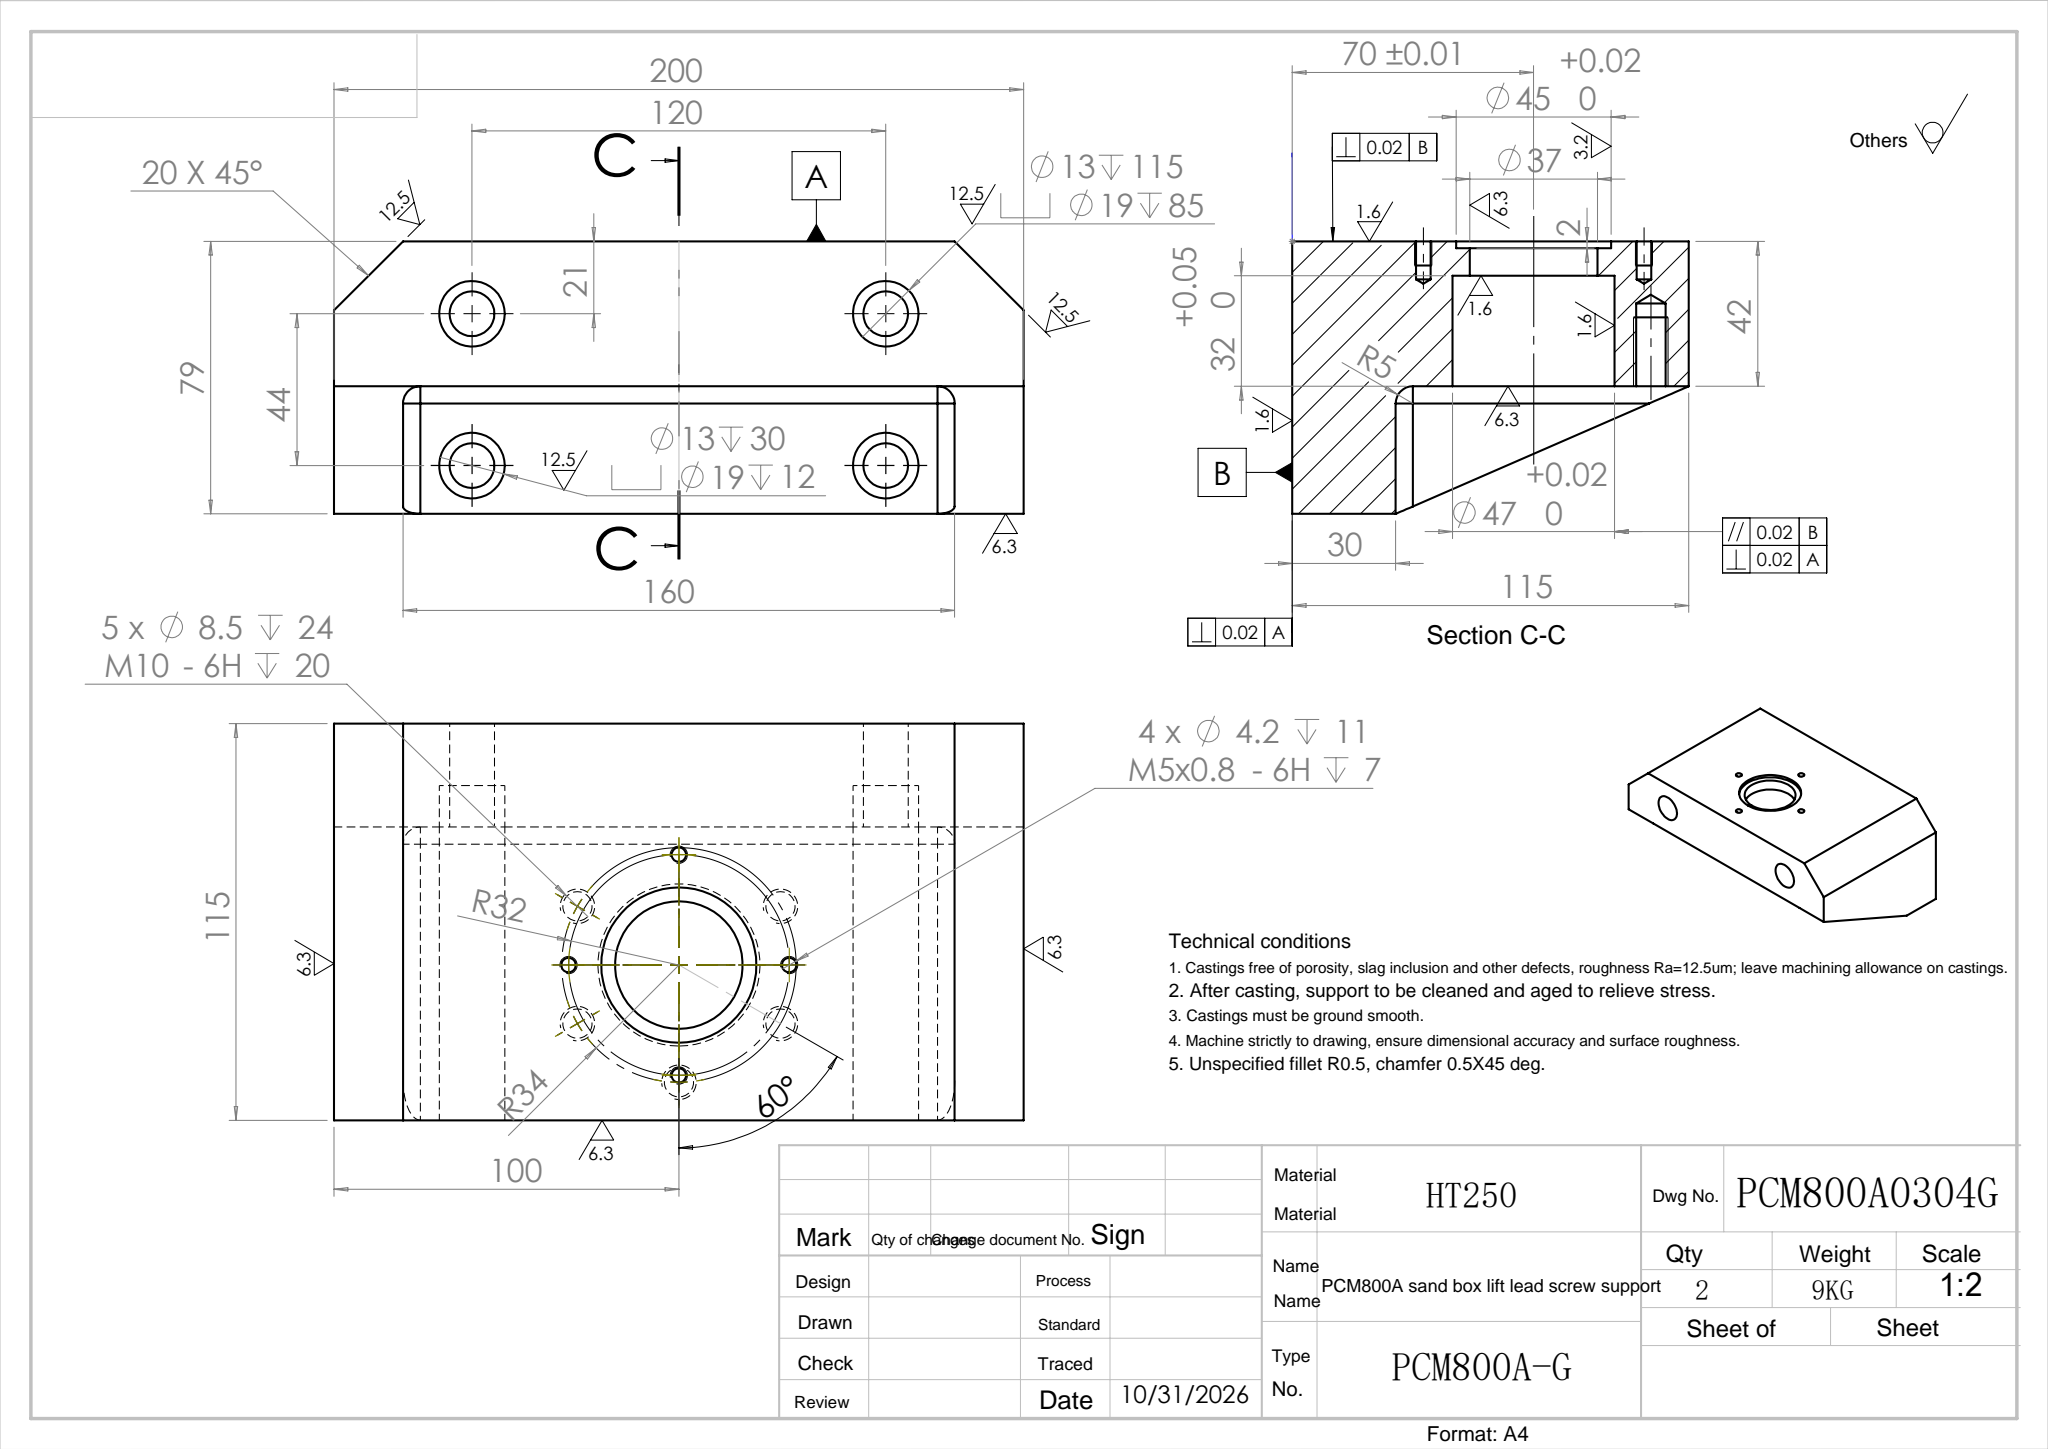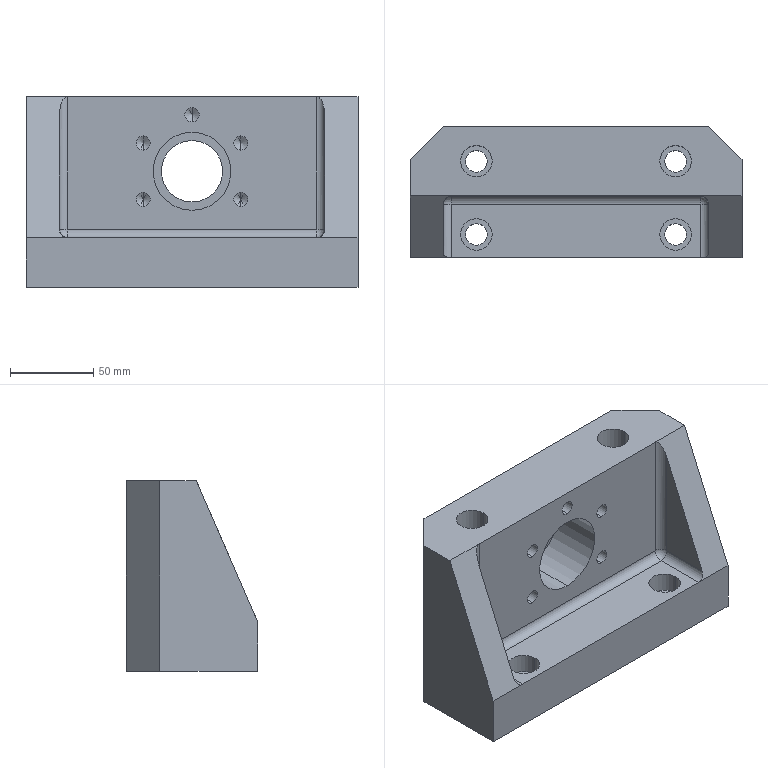Part | SolidWorks | features Cut 7, Boss 2, HoleWzd 2, ICE 2, Extrusion 1, Fillet 1, MirrorPattern 1 | 1 solid | 85 faces | box 200 x 79 x 115 mm | volume 1064261 mm3 | cylinder 45 | plane 20 | cone 18 | sphere 2 | commonest cylinder face diameters 8.5 x10 4.2 x8 13 x8 19 x8 10 x5 37 x2